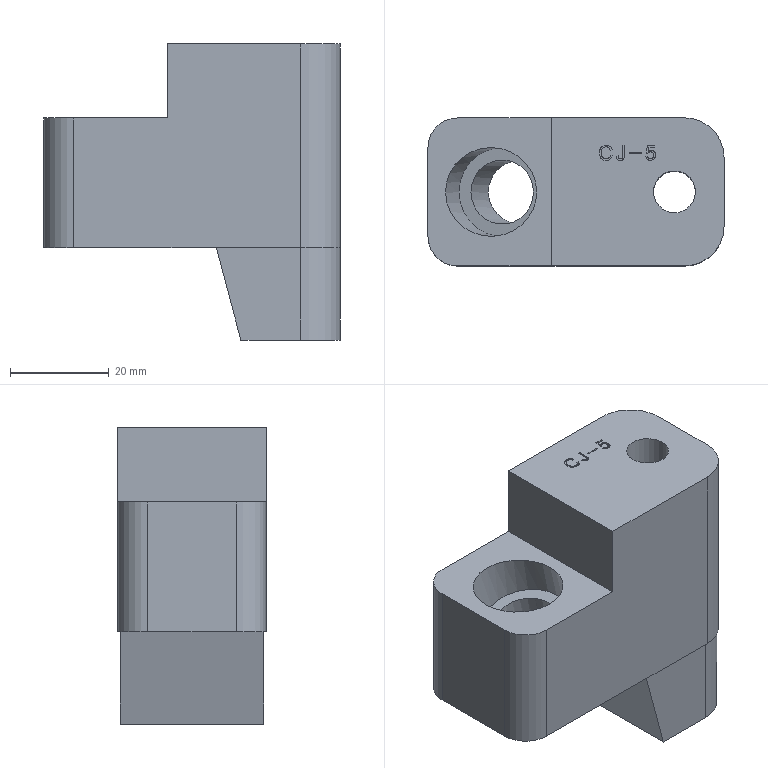Part | STEP file | solid 5 | 1 solid | 51 faces | box 60 x 30 x 60 mm | volume 64241 mm3 | plane 35 | cylinder 10 | other 6 | commonest cylinder face diameters 16 x4 12 x2 8.5 x1 13 x1 14 x1 18 x1